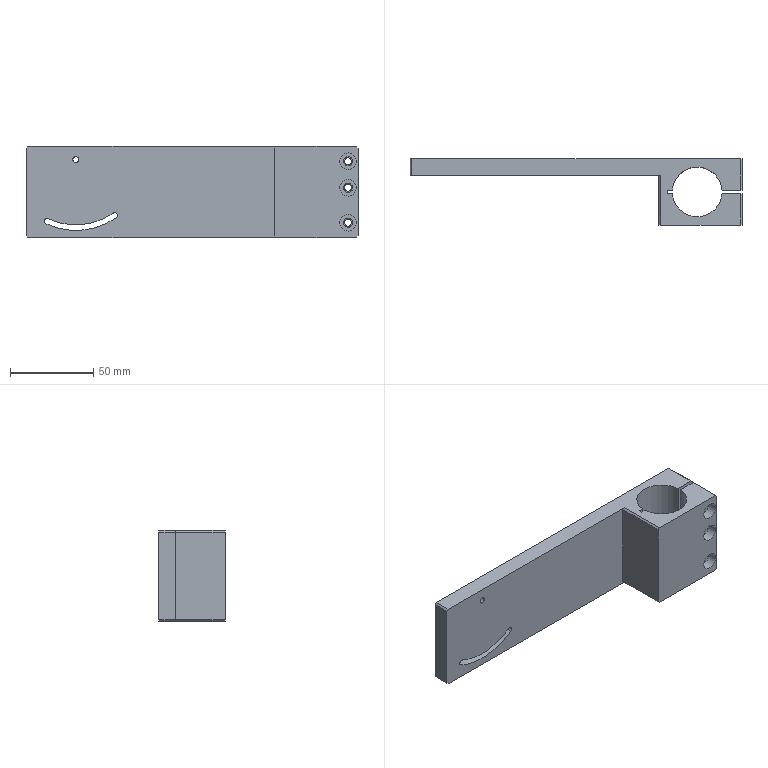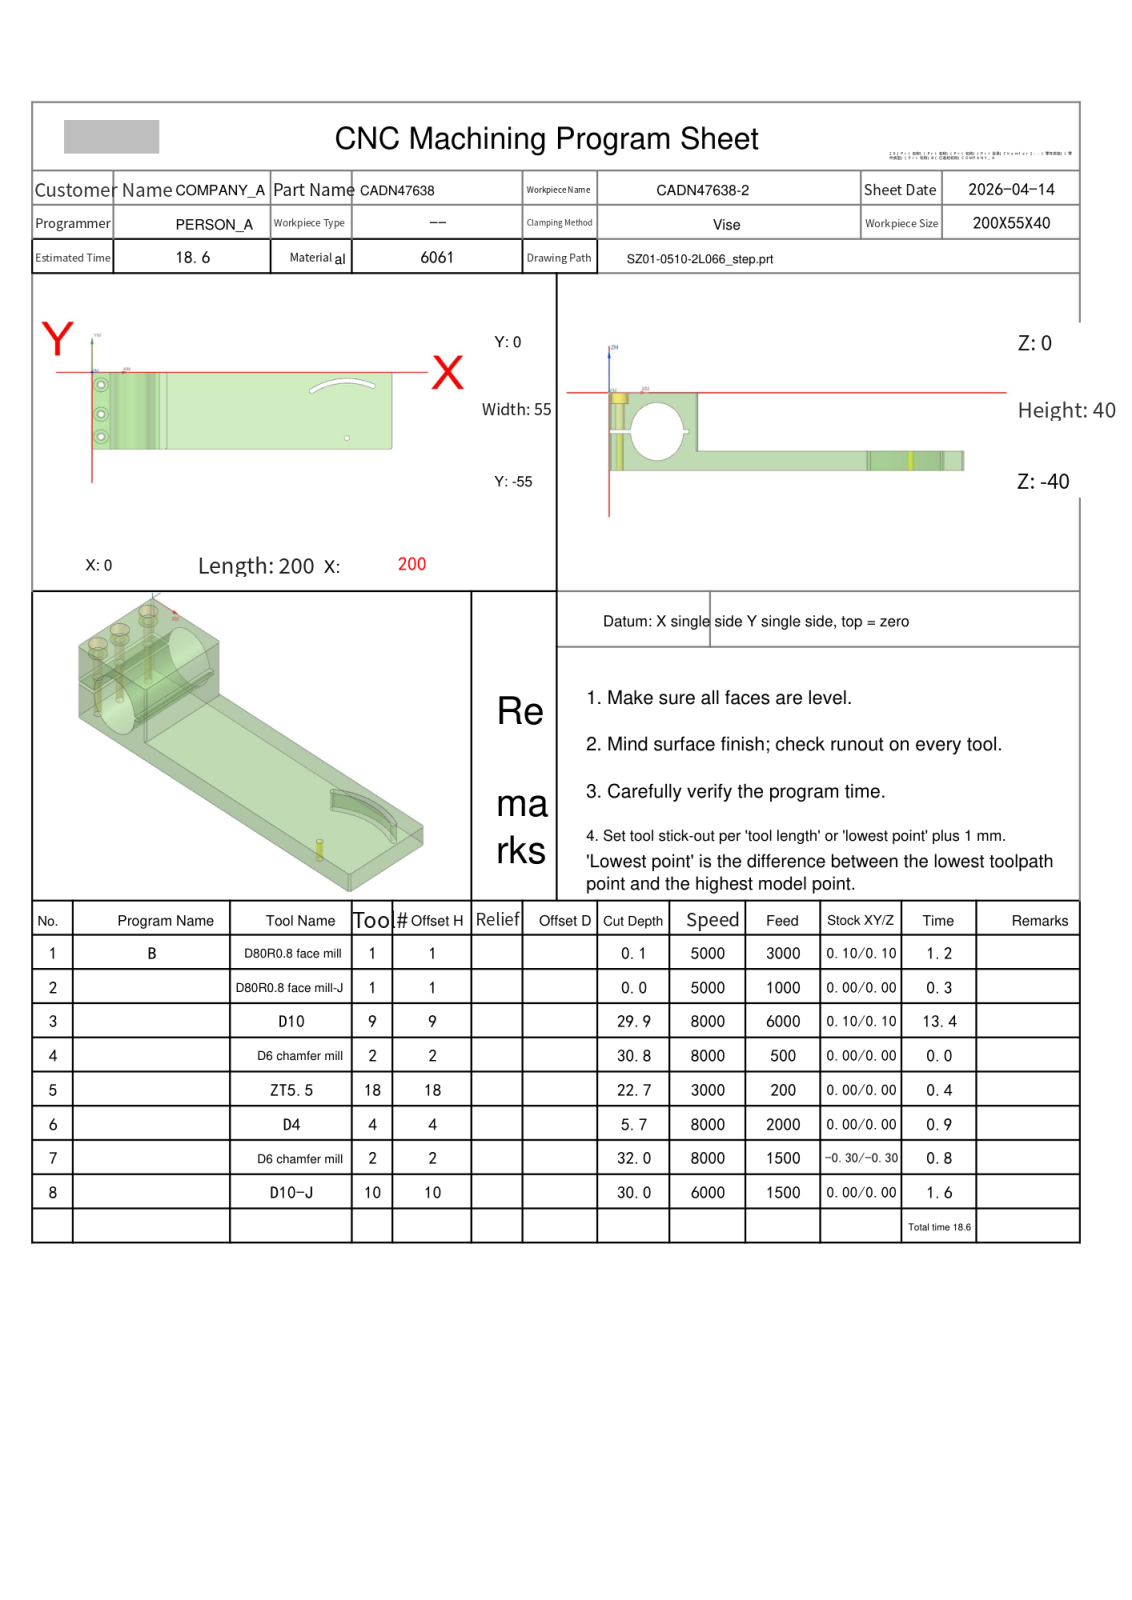NC program | NX | posted by the shop | part box 200 x 40 x 55 mm
Lines 1 to 112 of 8619:
%
O0001
(Machine time: 19.90 MIN)
(===Total Tool:6===)
(T1=D80R0.8 face mill D=80. R=0.8 D-H01 Z=-0.   )
(T9=D10     D=10.  R=0.   D-  H09 Z=-29.9 )
(T2=D6 chamfer mill D=6. R=0. D-H02 Z=-32.05)
(T18=ZT5.5  D=5.5  DR_a=118 D-  H18 Z=-22.65)
(T4=D4      D=4.   R=0.   D4  H04 Z=-5.7  )
(T10=D10-J  D=10.  R=0.   D10 H10 Z=-30.  )
G80 G90 G17 G49 G40
G91 G28 Z0
M01
N1 T01 M06
(D80R0.8 face mill D=80. R=0.8 H=01 ce=0.10 di=0.10)
(MAX_Z=20. MIN_Z=0.1 Time=1.10M)
G00 G90 G54 X-52.097 Y-27.5 M03 S5000
G43 H01 Z20.
M08
Z6.011
G01 Z4.011 F3000.
X-40.097
X240.097
X252.097
Z6.011
G00 X-52.097
Z5.522
G01 Z3.522
X-40.097
X240.097
X252.097
Z5.522
G00 X-52.097
Z5.033
G01 Z3.033
X-40.097
X240.097
X252.097
Z5.033
G00 X-52.097
Z4.544
G01 Z2.544
X-40.097
X240.097
X252.097
Z4.544
G00 Z20.
X-52.097
Z4.056
G01 Z2.056
X-40.097
X240.097
X252.097
Z4.056
G00 Z20.
X-52.097
Z3.567
G01 Z1.567
X-40.097
X240.097
X252.097
Z3.567
G00 Z20.
X-52.097
Z3.078
G01 Z1.078
X-40.097
X240.097
X252.097
Z3.078
G00 Z20.
X-52.097
Z2.589
G01 Z.589
X-40.097
X240.097
X252.097
Z2.589
G00 Z20.
X-52.097
Z2.1
G01 Z.1
X-40.097
X240.097
X252.097
Z2.1
G00 Z20.
G91 G28 Z0.0
M05
M09
G91 G28 Z0.0
M01
N2 T01 M06
(D80R0.8 face mill-J D=80. R=0.8 H=01 ce=0.00 di=0.00)
(MAX_Z=20. MIN_Z=-0. Time=0.33M)
G00 G90 G54 X-51.999 Y-27.5 M03 S5000
G43 H01 Z20.
M08
Z2.
G01 Z0.0 F1000.
X-39.999
X239.999
X251.999
Z2.
G00 Z20.
G91 G28 Z0.0
M05
M09
G91 G28 Z0.0
M01